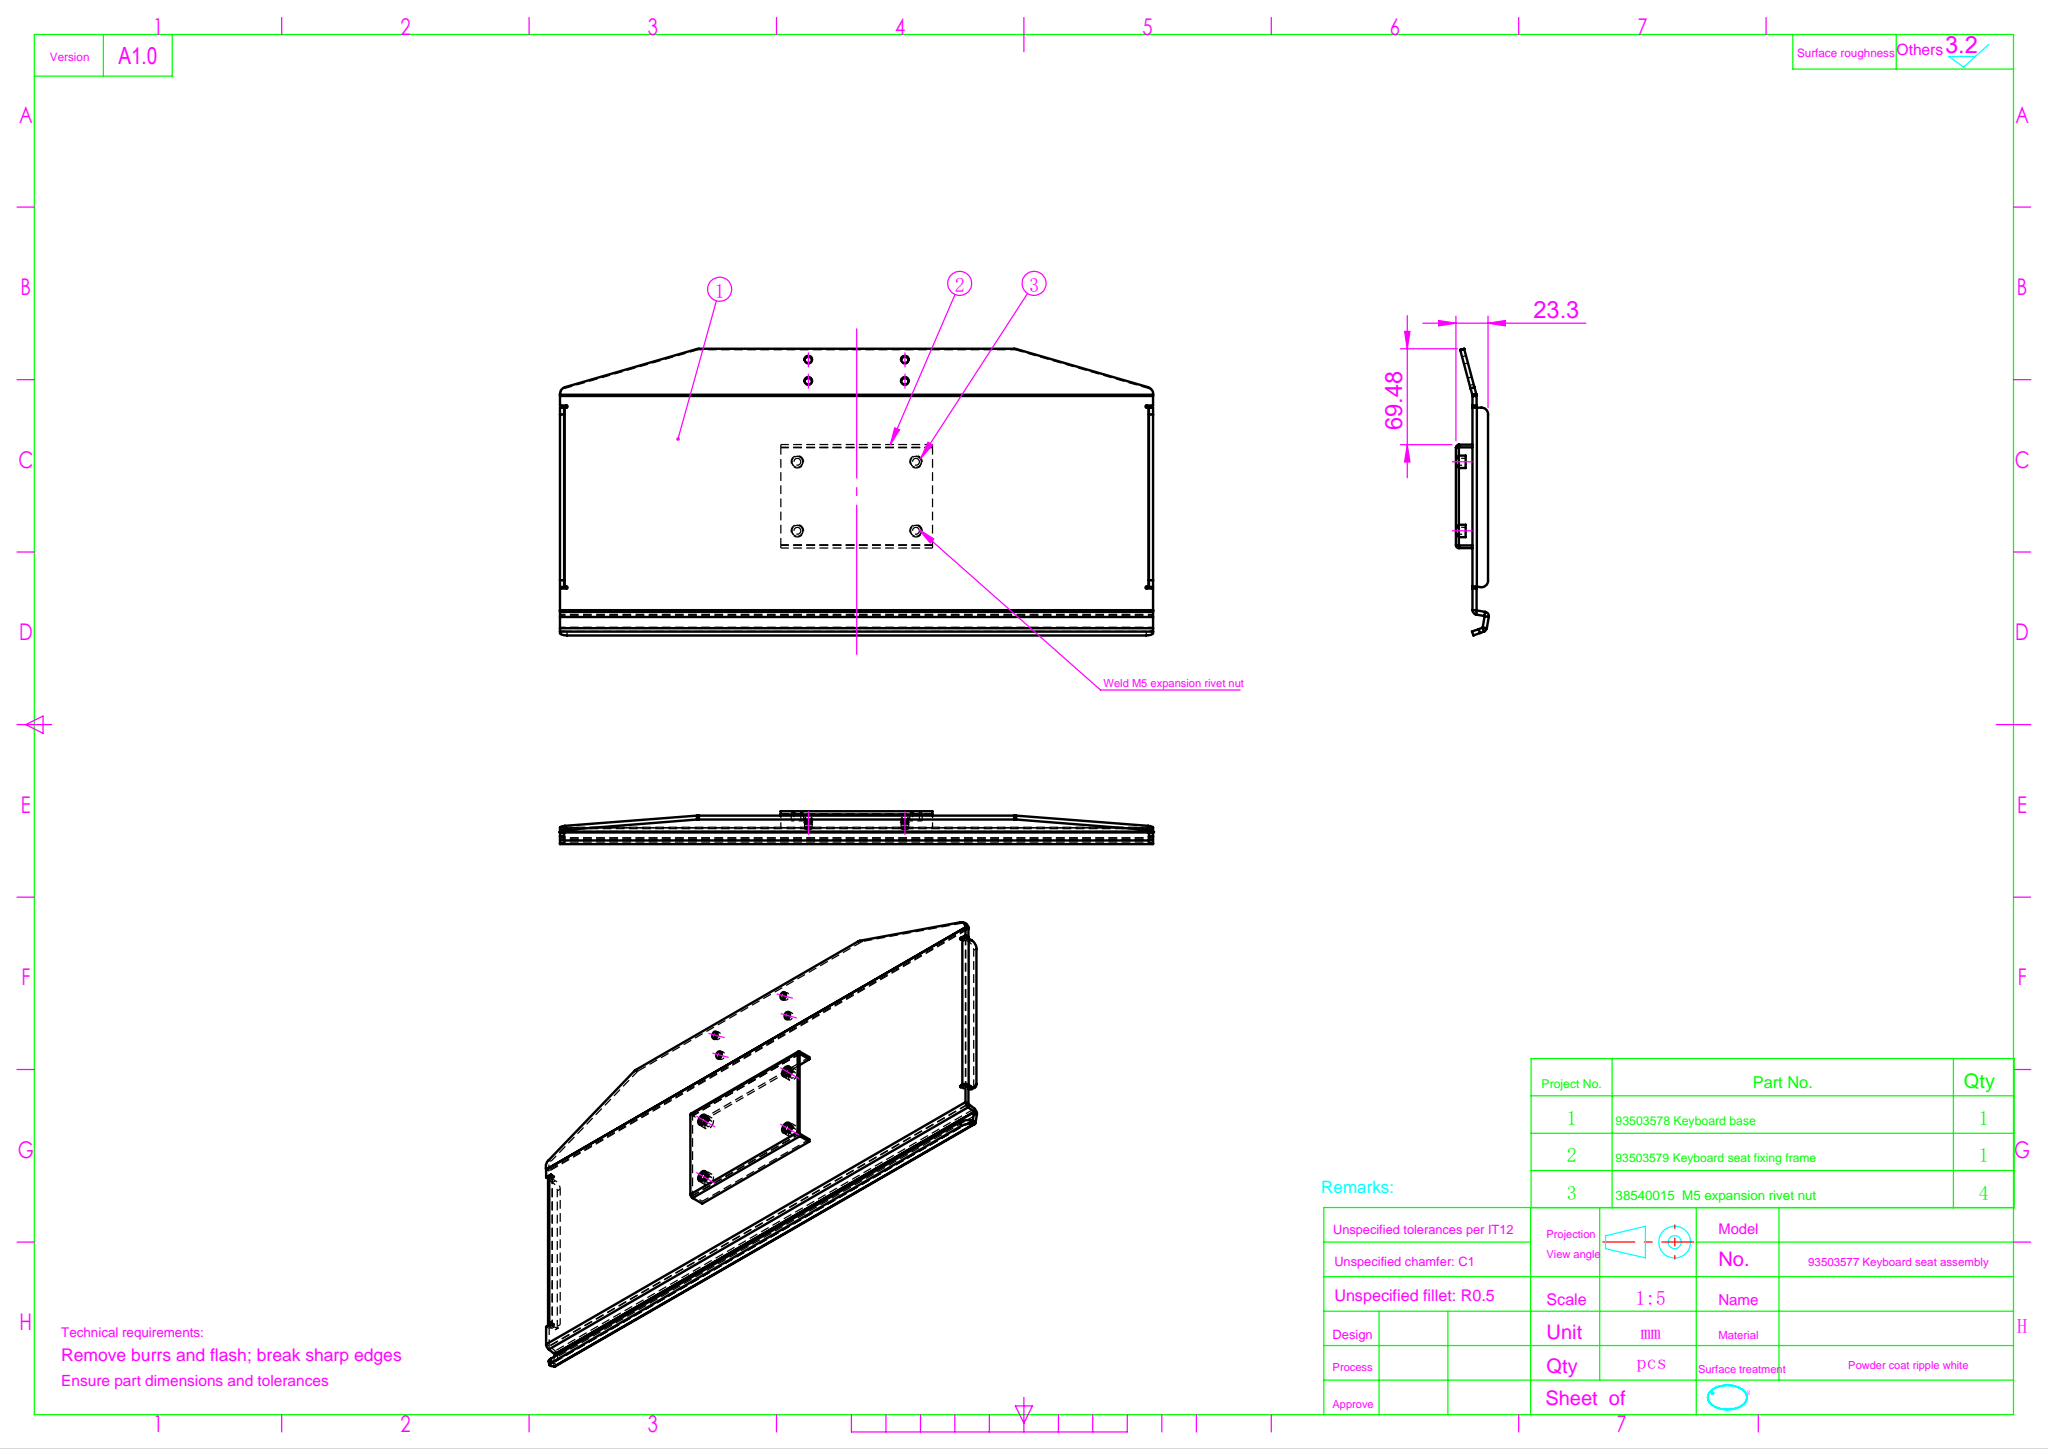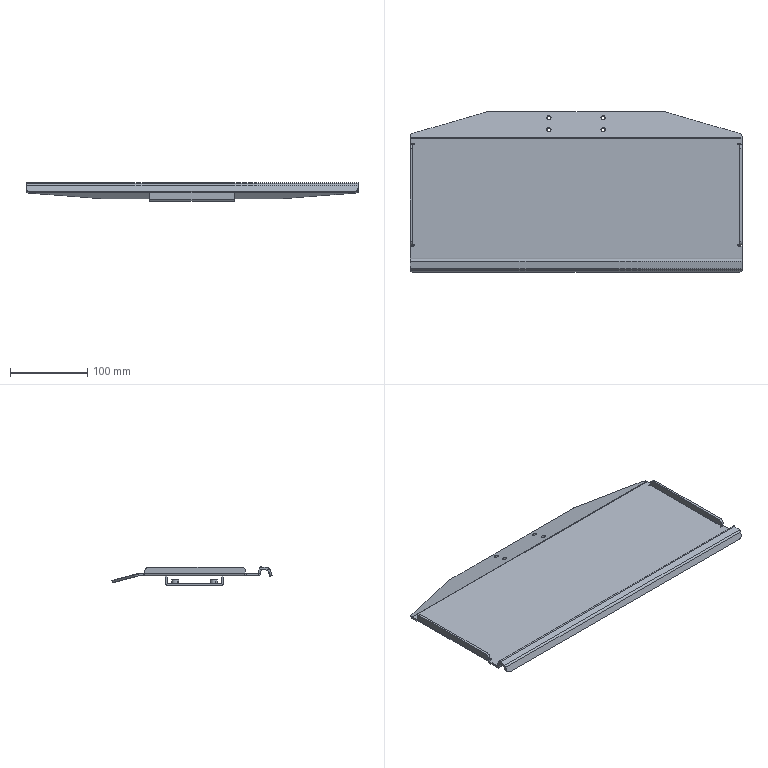Part | SolidWorks | 6 solids | 156 faces | box 430 x 207.698 x 23.832 mm | volume 300850 mm3 | plane 84 | cylinder 70 | spline 2 | commonest cylinder face diameters 8 x16 10 x10 0.4 x8 5 x8 5.5 x8 9 x8